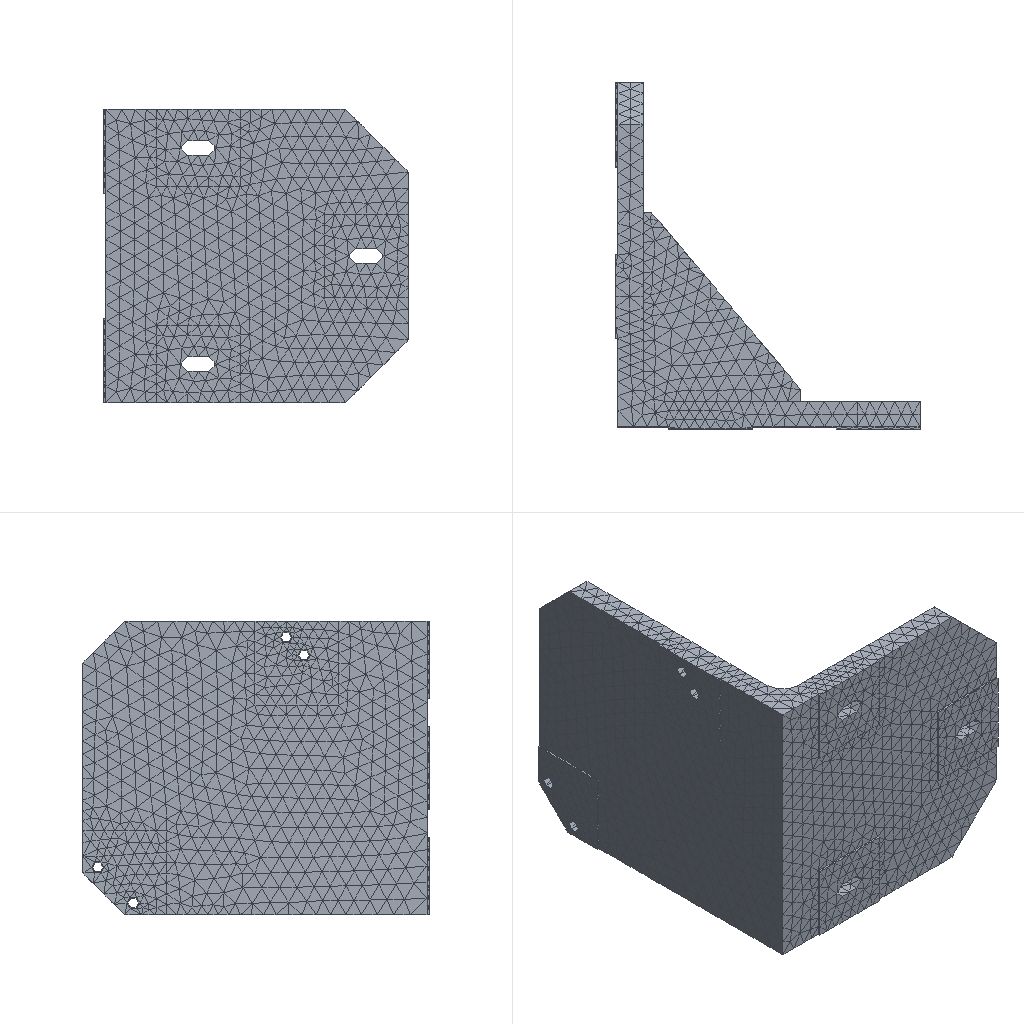Simulation study | nx simcenter
Set-up summary:
category,name,step,type,value,unit,region
solver,nx_nastran (Simcenter)
units,not stated in the deck,,not stated
analysis,deck,,static,static
analysis,solution,,SOL,101
load_step,SUBCASE 1,1,SUBCASE,SPC=1 LOAD=2
load_step,requested,,,1
mesh,nodes,,,20322
mesh,elements,,,11061
element_type,CTETRA,,solid,11061
load,nodal force total,,FX,-4999999.95,model units
load,nodal force total,,FY,0.0,model units
load,nodal force total,,FZ,0.0,model units
load,load commands in deck,,count,473
bc,support commands in deck,,count,692
analysis,NX solution 0,,Structural,Linear Statics - Single Constraint
check,setup vs results,,match,every grid point's frame and coordinates and every element id; grid points of CTETRA elements
Nastran input file, long lists of numbers shortened:
$*$$$$$$$$$$$$$$$$$$$$$$$$$$$$$$$$$$$$$$$$$$$$$$$$$$$$$$$$$$$$$$$$$
$*
$*                    NX v10.0.0.24 TRANSLATOR
$*                    FOR NX NASTRAN VERSION 10.0
$ (33 more lines like these left out)
ASSIGN OUTPUT2='111_sim1-solution_1.op2' UNIT=12
$*
$*$$$$$$$$$$$$$$$$$$$$$$$$$$$$$$$$$$$
$*
$* EXECUTIVE CONTROL
$*
$*$$$$$$$$$$$$$$$$$$$$$$$$$$$$$$$$$$$
$*
ID,NASTRAN,111_sim1-solution_1
SOL 101
CEND
$*
$*$$$$$$$$$$$$$$$$$$$$$$$$$$$$$$$$$$$
$*
$* CASE CONTROL
$*
$*$$$$$$$$$$$$$$$$$$$$$$$$$$$$$$$$$$$
$*
TITLE = Solution 1
ECHO = NONE
SPC = 1
OUTPUT
BCRESULTS(TRACTION,FORCE,PLOT) = ALL
DISPLACEMENT(PLOT) = ALL
ESE(PLOT) = ALL
FORCE(PLOT,CORNER) = ALL
OLOAD(PLOT) = ALL
SPCFORCES(PLOT) = ALL
STRAIN(PLOT,FIBER,CORNER) = ALL
STRESS(PLOT,CORNER) = ALL
$*  NX Step: Subcase - Static Loads 1
SUBCASE 1
LABEL = Subcase - Static Loads 1
LOAD = 2
$*
$*$$$$$$$$$$$$$$$$$$$$$$$$$$$$$$$$$$$
$*
$* BULK DATA
$*
$*$$$$$$$$$$$$$$$$$$$$$$$$$$$$$$$$$$$
$*
BEGIN BULK
$*
$* PARAM CARDS
$*
PARAM      K6ROT100.0000
PARAM     OIBULK     YES
PARAM    OMACHPR     YES
PARAM       POST      -2
PARAM    POSTEXT     YES
PARAM    UNITSYS   MN-MM
$*
$* GRID CARDS
$*
GRID*              20219               02.2043640700E-158.3000000000E+01+
*       1.4000000000E+02               0
GRID*              20220               02.2043640700E-158.3000000000E+01+
*       1.0000000000E+02               0
$ (40640 more lines like these left out)
$*
$* ELEMENT CARDS
$*
$*  NX Mesh Collector: Solid(1)
$*  NX Mesh: 3d_mesh(1)
CTETRA         1       1       1       2   17155   17158     583     584+
+            585     586     587   18265
CTETRA         2       1   20250   20163       3       1   20165     588+
+            589     590     591     592
$ (22118 more lines like these left out)
$*
$* PROPERTY CARDS
$*
$*  NX Property: PSOLID1
PSOLID         1       1       0                           SMECH
$*
$* MATERIAL CARDS
$*
$*  NX Material: Aluminum_A356
MAT1           17.0000+7        0.3300002.6700-62.1400-5
$*
$* LOAD AND CONSTRAINT CARDS
$*
$*  NX Load and Constraint: Fixed(1)
SPC            1   12894  123456  0.0000
SPC            1   12895  123456  0.0000
SPC            1   12896  123456  0.0000
SPC            1   12897  123456  0.0000
$ (688 more lines like these left out)
$*  NX Load and Constraint: Force(1)
FORCE          2   16401       0 2942.29-1.00000  0.0000  0.0000
FORCE          2   16402       0 3562.36-1.00000  0.0000  0.0000
FORCE          2   16403       0 4614.66-1.00000  0.0000  0.0000
FORCE          2   16404       0 3054.21-1.00000  0.0000  0.0000
$ (469 more lines like these left out)
ENDDATA 35c73097
Results summary:
result,analysis,,,static
result,last_loadstep,,,1
result,primary field,,,displacements
result,max displacement,,,0.6512,model units
result,reaction total,,FX,4999999.5,model units
result,reaction total,,FY,1.153,model units
result,reaction total,,FZ,0.03778,model units
result,NX solution 0,,loadcases,1,mm